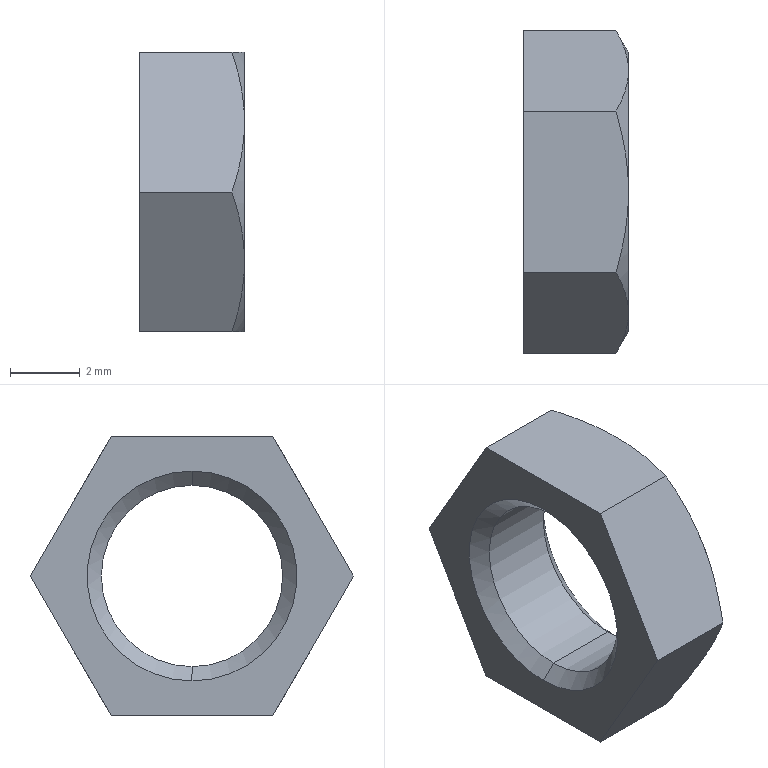Part | STEP file | 2_10 | 1 solid | 20 faces | box 3 x 9.238 x 8 mm | volume 99.469 mm3 | cone 10 | plane 8 | cylinder 2 | commonest cylinder face diameters 5.188 x2